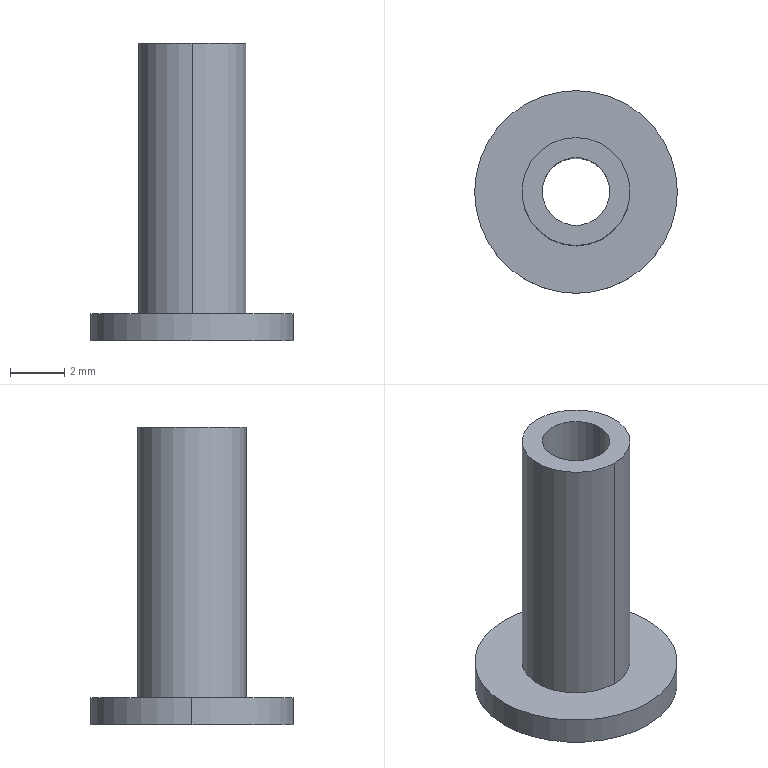Part | STEP file | High-temperature rubber spring guide shaft | 1 solid | 9 faces | box 7.5 x 7.5 x 11 mm | volume 115.846 mm3 | cylinder 6 | plane 3 | commonest cylinder face diameters 2.5 x2 4 x2 7.5 x2
STEP:
#1=CARTESIAN_POINT('',(0.,0.,0.));
#2=DIRECTION('',(0.,0.,1.));
#3=DIRECTION('',(1.,0.,0.));
#4=AXIS2_PLACEMENT_3D('',#1,#2,#3);
#5=CARTESIAN_POINT('',(-3.75,0.,-11.));
#6=VERTEX_POINT('',#5);
#7=CARTESIAN_POINT('',(3.75,0.,-11.));
#8=VERTEX_POINT('',#7);
#9=CARTESIAN_POINT('',(0.,0.,-11.));
#10=DIRECTION('',(0.,0.,-1.));
#11=DIRECTION('',(1.,0.,0.));
#12=AXIS2_PLACEMENT_3D('',#9,#10,#11);
#13=CIRCLE('',#12,3.75);
#14=CARTESIAN_POINT('',(0.,0.,-11.));
#15=DIRECTION('',(0.,0.,1.));
#16=DIRECTION('',(1.,0.,0.));
#17=AXIS2_PLACEMENT_3D('',#14,#15,#16);
#18=CYLINDRICAL_SURFACE('',#17,3.75);
#19=CARTESIAN_POINT('',(6.283,0.));
#20=DIRECTION('',(-1.,0.));
#21=VECTOR('',#20,1.);
#22=LINE('',#19,#21);
#23=(GEOMETRIC_REPRESENTATION_CONTEXT(2)PARAMETRIC_REPRESENTATION_CONTEXT()REPRESENTATION_CONTEXT('',''));
#24=DEFINITIONAL_REPRESENTATION('',(#22),#23);
#25=PCURVE('',#18,#24);
#26=CARTESIAN_POINT('',(-3.795,-3.795,-11.));
#27=DIRECTION('',(0.,0.,1.));
#28=DIRECTION('',(1.,0.,0.));
#29=AXIS2_PLACEMENT_3D('',#26,#27,#28);
#30=PLANE('',#29);
#31=CARTESIAN_POINT('',(7.545,3.795));
#32=CARTESIAN_POINT('',(7.545,-2.7));
#33=CARTESIAN_POINT('',(1.92,0.5474));
#34=CARTESIAN_POINT('',(-3.705,3.795));
#35=CARTESIAN_POINT('',(1.92,7.043));
#36=CARTESIAN_POINT('',(7.545,10.29));
#37=CARTESIAN_POINT('',(7.545,3.795));
#38=(BOUNDED_CURVE()B_SPLINE_CURVE(2,(#31,#32,#33,#34,#35,#36,#37),.UNSPECIFIED.,.T.,.F.)B_SPLINE_CURVE_WITH_KNOTS((1,2,2,2,2,1),(-2.094,0.,2.094,4.189,6.283,8.378),.UNSPECIFIED.)CURVE()GEOMETRIC_REPRESENTATION_ITEM()RATIONAL_B_SPLINE_CURVE((1.,0.5,1.,0.5,1.,0.5,1.))REPRESENTATION_ITEM(''));
#39=(GEOMETRIC_REPRESENTATION_CONTEXT(2)PARAMETRIC_REPRESENTATION_CONTEXT()REPRESENTATION_CONTEXT('',''));
#40=DEFINITIONAL_REPRESENTATION('',(#38),#39);
#41=PCURVE('',#30,#40);
#42=SURFACE_CURVE('',#13,(#25,#41),.PCURVE_S1.);
#43=EDGE_CURVE('',#6,#8,#42,.T.);
#44=ORIENTED_EDGE('',*,*,#43,.F.);
#45=CARTESIAN_POINT('',(-3.75,0.,-10.));
#46=VERTEX_POINT('',#45);
#47=CARTESIAN_POINT('',(-3.75,0.,-11.));
#48=DIRECTION('',(0.,0.,1.));
#49=VECTOR('',#48,1.);
#50=LINE('',#47,#49);
#51=CARTESIAN_POINT('',(3.142,0.));
#52=DIRECTION('',(0.,1.));
#53=VECTOR('',#52,1.);
#54=LINE('',#51,#53);
#55=(GEOMETRIC_REPRESENTATION_CONTEXT(2)PARAMETRIC_REPRESENTATION_CONTEXT()REPRESENTATION_CONTEXT('',''));
#56=DEFINITIONAL_REPRESENTATION('',(#54),#55);
#57=PCURVE('',#18,#56);
#58=CARTESIAN_POINT('',(0.,0.,-11.));
#59=DIRECTION('',(0.,0.,1.));
#60=DIRECTION('',(1.,0.,0.));
#61=AXIS2_PLACEMENT_3D('',#58,#59,#60);
#62=CYLINDRICAL_SURFACE('',#61,3.75);
#63=CARTESIAN_POINT('',(3.142,0.));
#64=DIRECTION('',(0.,1.));
#65=VECTOR('',#64,1.);
#66=LINE('',#63,#65);
#67=(GEOMETRIC_REPRESENTATION_CONTEXT(2)PARAMETRIC_REPRESENTATION_CONTEXT()REPRESENTATION_CONTEXT('',''));
#68=DEFINITIONAL_REPRESENTATION('',(#66),#67);
#69=PCURVE('',#62,#68);
#70=SURFACE_CURVE('',#50,(#57,#69),.PCURVE_S1.);
#71=EDGE_CURVE('',#6,#46,#70,.T.);
#72=ORIENTED_EDGE('',*,*,#71,.T.);
#73=CARTESIAN_POINT('',(3.75,0.,-10.));
#74=VERTEX_POINT('',#73);
#75=CARTESIAN_POINT('',(0.,0.,-10.));
#76=DIRECTION('',(0.,0.,1.));
#77=DIRECTION('',(1.,0.,0.));
#78=AXIS2_PLACEMENT_3D('',#75,#76,#77);
#79=CIRCLE('',#78,3.75);
#80=CARTESIAN_POINT('',(0.,1.));
#81=DIRECTION('',(1.,0.));
#82=VECTOR('',#81,1.);
#83=LINE('',#80,#82);
#84=(GEOMETRIC_REPRESENTATION_CONTEXT(2)PARAMETRIC_REPRESENTATION_CONTEXT()REPRESENTATION_CONTEXT('',''));
#85=DEFINITIONAL_REPRESENTATION('',(#83),#84);
#86=PCURVE('',#18,#85);
#87=CARTESIAN_POINT('',(3.795,-3.795,-10.));
#88=DIRECTION('',(0.,0.,-1.));
#89=DIRECTION('',(-1.,0.,0.));
#90=AXIS2_PLACEMENT_3D('',#87,#88,#89);
#91=PLANE('',#90);
#92=CARTESIAN_POINT('',(0.045,3.795));
#93=CARTESIAN_POINT('',(0.045,10.29));
#94=CARTESIAN_POINT('',(5.67,7.043));
#95=CARTESIAN_POINT('',(11.295,3.795));
#96=CARTESIAN_POINT('',(5.67,0.5474));
#97=CARTESIAN_POINT('',(0.045,-2.7));
#98=CARTESIAN_POINT('',(0.045,3.795));
#99=(BOUNDED_CURVE()B_SPLINE_CURVE(2,(#92,#93,#94,#95,#96,#97,#98),.UNSPECIFIED.,.T.,.F.)B_SPLINE_CURVE_WITH_KNOTS((1,2,2,2,2,1),(-2.094,0.,2.094,4.189,6.283,8.378),.UNSPECIFIED.)CURVE()GEOMETRIC_REPRESENTATION_ITEM()RATIONAL_B_SPLINE_CURVE((1.,0.5,1.,0.5,1.,0.5,1.))REPRESENTATION_ITEM(''));
#100=(GEOMETRIC_REPRESENTATION_CONTEXT(2)PARAMETRIC_REPRESENTATION_CONTEXT()REPRESENTATION_CONTEXT('',''));
#101=DEFINITIONAL_REPRESENTATION('',(#99),#100);
#102=PCURVE('',#91,#101);
#103=SURFACE_CURVE('',#79,(#86,#102),.PCURVE_S1.);
#104=EDGE_CURVE('',#74,#46,#103,.T.);
#105=ORIENTED_EDGE('',*,*,#104,.F.);
#106=CARTESIAN_POINT('',(3.75,0.,-11.));
#107=DIRECTION('',(0.,0.,1.));
#108=VECTOR('',#107,1.);
#109=LINE('',#106,#108);
#110=CARTESIAN_POINT('',(0.,0.));
#111=DIRECTION('',(0.,1.));
#112=VECTOR('',#111,1.);
#113=LINE('',#110,#112);
#114=(GEOMETRIC_REPRESENTATION_CONTEXT(2)PARAMETRIC_REPRESENTATION_CONTEXT()REPRESENTATION_CONTEXT('',''));
#115=DEFINITIONAL_REPRESENTATION('',(#113),#114);
#116=PCURVE('',#18,#115);
#117=CARTESIAN_POINT('',(6.283,0.));
#118=DIRECTION('',(0.,1.));
#119=VECTOR('',#118,1.);
#120=LINE('',#117,#119);
#121=(GEOMETRIC_REPRESENTATION_CONTEXT(2)PARAMETRIC_REPRESENTATION_CONTEXT()REPRESENTATION_CONTEXT('',''));
#122=DEFINITIONAL_REPRESENTATION('',(#120),#121);
#123=PCURVE('',#62,#122);
#124=SURFACE_CURVE('',#109,(#116,#123),.PCURVE_S1.);
#125=EDGE_CURVE('',#8,#74,#124,.T.);
#126=ORIENTED_EDGE('',*,*,#125,.F.);
#127=EDGE_LOOP('',(#44,#72,#105,#126));
#128=FACE_BOUND('',#127,.T.);
#129=ADVANCED_FACE('',(#128),#18,.T.);
#130=CARTESIAN_POINT('',(1.25,0.,-11.));
#131=VERTEX_POINT('',#130);
#132=CARTESIAN_POINT('',(1.25,0.,0.));
#133=VERTEX_POINT('',#132);
#134=CARTESIAN_POINT('',(1.25,0.,-11.));
#135=DIRECTION('',(0.,0.,1.));
#136=VECTOR('',#135,1.);
#137=LINE('',#134,#136);
#138=CARTESIAN_POINT('',(0.,0.,-11.));
#139=DIRECTION('',(0.,0.,1.));
#140=DIRECTION('',(1.,0.,0.));
#141=AXIS2_PLACEMENT_3D('',#138,#139,#140);
#142=CYLINDRICAL_SURFACE('',#141,1.25);
#143=CARTESIAN_POINT('',(6.283,0.));
#144=DIRECTION('',(0.,1.));
#145=VECTOR('',#144,1.);
#146=LINE('',#143,#145);
#147=(GEOMETRIC_REPRESENTATION_CONTEXT(2)PARAMETRIC_REPRESENTATION_CONTEXT()REPRESENTATION_CONTEXT('',''));
#148=DEFINITIONAL_REPRESENTATION('',(#146),#147);
#149=PCURVE('',#142,#148);
#150=CARTESIAN_POINT('',(0.,0.,-11.));
#151=DIRECTION('',(0.,0.,1.));
#152=DIRECTION('',(1.,0.,0.));
#153=AXIS2_PLACEMENT_3D('',#150,#151,#152);
#154=CYLINDRICAL_SURFACE('',#153,1.25);
#155=CARTESIAN_POINT('',(0.,0.));
#156=DIRECTION('',(0.,1.));
#157=VECTOR('',#156,1.);
#158=LINE('',#155,#157);
#159=(GEOMETRIC_REPRESENTATION_CONTEXT(2)PARAMETRIC_REPRESENTATION_CONTEXT()REPRESENTATION_CONTEXT('',''));
#160=DEFINITIONAL_REPRESENTATION('',(#158),#159);
#161=PCURVE('',#154,#160);
#162=SURFACE_CURVE('',#137,(#149,#161),.PCURVE_S1.);
#163=EDGE_CURVE('',#131,#133,#162,.T.);
#164=ORIENTED_EDGE('',*,*,#163,.T.);
#165=CARTESIAN_POINT('',(-1.25,0.,0.));
#166=VERTEX_POINT('',#165);
#167=CARTESIAN_POINT('',(0.,0.,0.));
#168=DIRECTION('',(0.,0.,1.));
#169=DIRECTION('',(1.,0.,0.));
#170=AXIS2_PLACEMENT_3D('',#167,#168,#169);
#171=CIRCLE('',#170,1.25);
#172=CARTESIAN_POINT('',(0.,11.));
#173=DIRECTION('',(1.,0.));
#174=VECTOR('',#173,1.);
#175=LINE('',#172,#174);
#176=(GEOMETRIC_REPRESENTATION_CONTEXT(2)PARAMETRIC_REPRESENTATION_CONTEXT()REPRESENTATION_CONTEXT('',''));
#177=DEFINITIONAL_REPRESENTATION('',(#175),#176);
#178=PCURVE('',#142,#177);
#179=CARTESIAN_POINT('',(2.024,-2.024,0.));
#180=DIRECTION('',(0.,0.,-1.));
#181=DIRECTION('',(-1.,0.,0.));
#182=AXIS2_PLACEMENT_3D('',#179,#180,#181);
#183=PLANE('',#182);
#184=CARTESIAN_POINT('',(0.774,2.024));
#185=CARTESIAN_POINT('',(0.774,4.189));
#186=CARTESIAN_POINT('',(2.649,3.107));
#187=CARTESIAN_POINT('',(4.524,2.024));
#188=CARTESIAN_POINT('',(2.649,0.9415));
#189=CARTESIAN_POINT('',(0.774,-0.1411));
#190=CARTESIAN_POINT('',(0.774,2.024));
#191=(BOUNDED_CURVE()B_SPLINE_CURVE(2,(#184,#185,#186,#187,#188,#189,#190),.UNSPECIFIED.,.T.,.F.)B_SPLINE_CURVE_WITH_KNOTS((1,2,2,2,2,1),(-2.094,0.,2.094,4.189,6.283,8.378),.UNSPECIFIED.)CURVE()GEOMETRIC_REPRESENTATION_ITEM()RATIONAL_B_SPLINE_CURVE((1.,0.5,1.,0.5,1.,0.5,1.))REPRESENTATION_ITEM(''));
#192=(GEOMETRIC_REPRESENTATION_CONTEXT(2)PARAMETRIC_REPRESENTATION_CONTEXT()REPRESENTATION_CONTEXT('',''));
#193=DEFINITIONAL_REPRESENTATION('',(#191),#192);
#194=PCURVE('',#183,#193);
#195=SURFACE_CURVE('',#171,(#178,#194),.PCURVE_S1.);
#196=EDGE_CURVE('',#166,#133,#195,.T.);
#197=ORIENTED_EDGE('',*,*,#196,.F.);
#198=CARTESIAN_POINT('',(-1.25,0.,-11.));
#199=VERTEX_POINT('',#198);
#200=CARTESIAN_POINT('',(-1.25,0.,-11.));
#201=DIRECTION('',(0.,0.,1.));
#202=VECTOR('',#201,1.);
#203=LINE('',#200,#202);
#204=CARTESIAN_POINT('',(3.142,0.));
#205=DIRECTION('',(0.,1.));
#206=VECTOR('',#205,1.);
#207=LINE('',#204,#206);
#208=(GEOMETRIC_REPRESENTATION_CONTEXT(2)PARAMETRIC_REPRESENTATION_CONTEXT()REPRESENTATION_CONTEXT('',''));
#209=DEFINITIONAL_REPRESENTATION('',(#207),#208);
#210=PCURVE('',#142,#209);
#211=CARTESIAN_POINT('',(3.142,0.));
#212=DIRECTION('',(0.,1.));
#213=VECTOR('',#212,1.);
#214=LINE('',#211,#213);
#215=(GEOMETRIC_REPRESENTATION_CONTEXT(2)PARAMETRIC_REPRESENTATION_CONTEXT()REPRESENTATION_CONTEXT('',''));
#216=DEFINITIONAL_REPRESENTATION('',(#214),#215);
#217=PCURVE('',#154,#216);
#218=SURFACE_CURVE('',#203,(#210,#217),.PCURVE_S1.);
#219=EDGE_CURVE('',#199,#166,#218,.T.);
#220=ORIENTED_EDGE('',*,*,#219,.F.);
#221=CARTESIAN_POINT('',(0.,0.,-11.));
#222=DIRECTION('',(0.,0.,-1.));
#223=DIRECTION('',(1.,0.,0.));
#224=AXIS2_PLACEMENT_3D('',#221,#222,#223);
#225=CIRCLE('',#224,1.25);
#226=CARTESIAN_POINT('',(6.283,0.));
#227=DIRECTION('',(-1.,0.));
#228=VECTOR('',#227,1.);
#229=LINE('',#226,#228);
#230=(GEOMETRIC_REPRESENTATION_CONTEXT(2)PARAMETRIC_REPRESENTATION_CONTEXT()REPRESENTATION_CONTEXT('',''));
#231=DEFINITIONAL_REPRESENTATION('',(#229),#230);
#232=PCURVE('',#142,#231);
#233=CARTESIAN_POINT('',(5.045,3.795));
#234=CARTESIAN_POINT('',(5.045,1.63));
#235=CARTESIAN_POINT('',(3.17,2.712));
#236=CARTESIAN_POINT('',(1.295,3.795));
#237=CARTESIAN_POINT('',(3.17,4.878));
#238=CARTESIAN_POINT('',(5.045,5.96));
#239=CARTESIAN_POINT('',(5.045,3.795));
#240=(BOUNDED_CURVE()B_SPLINE_CURVE(2,(#233,#234,#235,#236,#237,#238,#239),.UNSPECIFIED.,.T.,.F.)B_SPLINE_CURVE_WITH_KNOTS((1,2,2,2,2,1),(-2.094,0.,2.094,4.189,6.283,8.378),.UNSPECIFIED.)CURVE()GEOMETRIC_REPRESENTATION_ITEM()RATIONAL_B_SPLINE_CURVE((1.,0.5,1.,0.5,1.,0.5,1.))REPRESENTATION_ITEM(''));
#241=(GEOMETRIC_REPRESENTATION_CONTEXT(2)PARAMETRIC_REPRESENTATION_CONTEXT()REPRESENTATION_CONTEXT('',''));
#242=DEFINITIONAL_REPRESENTATION('',(#240),#241);
#243=PCURVE('',#30,#242);
#244=SURFACE_CURVE('',#225,(#232,#243),.PCURVE_S1.);
#245=EDGE_CURVE('',#131,#199,#244,.T.);
#246=ORIENTED_EDGE('',*,*,#245,.F.);
#247=EDGE_LOOP('',(#164,#197,#220,#246));
#248=FACE_BOUND('',#247,.F.);
#249=ADVANCED_FACE('',(#248),#142,.F.);
#250=CARTESIAN_POINT('',(0.,-2.,-10.));
#251=VERTEX_POINT('',#250);
#252=CARTESIAN_POINT('',(0.,2.,-10.));
#253=VERTEX_POINT('',#252);
#254=CARTESIAN_POINT('',(0.,0.,-10.));
#255=DIRECTION('',(0.,0.,1.));
#256=DIRECTION('',(0.,-1.,0.));
#257=AXIS2_PLACEMENT_3D('',#254,#255,#256);
#258=CIRCLE('',#257,2.);
#259=CARTESIAN_POINT('',(0.,0.,-10.));
#260=DIRECTION('',(0.,0.,1.));
#261=DIRECTION('',(0.,-1.,0.));
#262=AXIS2_PLACEMENT_3D('',#259,#260,#261);
#263=CYLINDRICAL_SURFACE('',#262,2.);
#264=CARTESIAN_POINT('',(0.,0.));
#265=DIRECTION('',(1.,0.));
#266=VECTOR('',#265,1.);
#267=LINE('',#264,#266);
#268=(GEOMETRIC_REPRESENTATION_CONTEXT(2)PARAMETRIC_REPRESENTATION_CONTEXT()REPRESENTATION_CONTEXT('',''));
#269=DEFINITIONAL_REPRESENTATION('',(#267),#268);
#270=PCURVE('',#263,#269);
#271=CARTESIAN_POINT('',(3.795,1.795));
#272=CARTESIAN_POINT('',(0.3309,1.795));
#273=CARTESIAN_POINT('',(2.063,4.795));
#274=CARTESIAN_POINT('',(3.795,7.795));
#275=CARTESIAN_POINT('',(5.527,4.795));
#276=CARTESIAN_POINT('',(7.259,1.795));
#277=CARTESIAN_POINT('',(3.795,1.795));
#278=(BOUNDED_CURVE()B_SPLINE_CURVE(2,(#271,#272,#273,#274,#275,#276,#277),.UNSPECIFIED.,.T.,.F.)B_SPLINE_CURVE_WITH_KNOTS((1,2,2,2,2,1),(-2.094,0.,2.094,4.189,6.283,8.378),.UNSPECIFIED.)CURVE()GEOMETRIC_REPRESENTATION_ITEM()RATIONAL_B_SPLINE_CURVE((1.,0.5,1.,0.5,1.,0.5,1.))REPRESENTATION_ITEM(''));
#279=(GEOMETRIC_REPRESENTATION_CONTEXT(2)PARAMETRIC_REPRESENTATION_CONTEXT()REPRESENTATION_CONTEXT('',''));
#280=DEFINITIONAL_REPRESENTATION('',(#278),#279);
#281=PCURVE('',#91,#280);
#282=SURFACE_CURVE('',#258,(#270,#281),.PCURVE_S1.);
#283=EDGE_CURVE('',#251,#253,#282,.T.);
#284=ORIENTED_EDGE('',*,*,#283,.T.);
#285=CARTESIAN_POINT('',(0.,2.,0.));
#286=VERTEX_POINT('',#285);
#287=CARTESIAN_POINT('',(0.,2.,-10.));
#288=DIRECTION('',(0.,0.,1.));
#289=VECTOR('',#288,1.);
#290=LINE('',#287,#289);
#291=CARTESIAN_POINT('',(3.142,0.));
#292=DIRECTION('',(0.,1.));
#293=VECTOR('',#292,1.);
#294=LINE('',#291,#293);
#295=(GEOMETRIC_REPRESENTATION_CONTEXT(2)PARAMETRIC_REPRESENTATION_CONTEXT()REPRESENTATION_CONTEXT('',''));
#296=DEFINITIONAL_REPRESENTATION('',(#294),#295);
#297=PCURVE('',#263,#296);
#298=CARTESIAN_POINT('',(0.,0.,-10.));
#299=DIRECTION('',(0.,0.,1.));
#300=DIRECTION('',(0.,-1.,0.));
#301=AXIS2_PLACEMENT_3D('',#298,#299,#300);
#302=CYLINDRICAL_SURFACE('',#301,2.);
#303=CARTESIAN_POINT('',(3.142,0.));
#304=DIRECTION('',(0.,1.));
#305=VECTOR('',#304,1.);
#306=LINE('',#303,#305);
#307=(GEOMETRIC_REPRESENTATION_CONTEXT(2)PARAMETRIC_REPRESENTATION_CONTEXT()REPRESENTATION_CONTEXT('',''));
#308=DEFINITIONAL_REPRESENTATION('',(#306),#307);
#309=PCURVE('',#302,#308);
#310=SURFACE_CURVE('',#290,(#297,#309),.PCURVE_S1.);
#311=EDGE_CURVE('',#253,#286,#310,.T.);
#312=ORIENTED_EDGE('',*,*,#311,.T.);
#313=CARTESIAN_POINT('',(0.,-2.,0.));
#314=VERTEX_POINT('',#313);
#315=CARTESIAN_POINT('',(0.,0.,0.));
#316=DIRECTION('',(0.,0.,1.));
#317=DIRECTION('',(0.,-1.,0.));
#318=AXIS2_PLACEMENT_3D('',#315,#316,#317);
#319=CIRCLE('',#318,2.);
#320=CARTESIAN_POINT('',(0.,10.));
#321=DIRECTION('',(1.,0.));
#322=VECTOR('',#321,1.);
#323=LINE('',#320,#322);
#324=(GEOMETRIC_REPRESENTATION_CONTEXT(2)PARAMETRIC_REPRESENTATION_CONTEXT()REPRESENTATION_CONTEXT('',''));
#325=DEFINITIONAL_REPRESENTATION('',(#323),#324);
#326=PCURVE('',#263,#325);
#327=CARTESIAN_POINT('',(2.024,0.024));
#328=CARTESIAN_POINT('',(-1.44,0.024));
#329=CARTESIAN_POINT('',(0.2919,3.024));
#330=CARTESIAN_POINT('',(2.024,6.024));
#331=CARTESIAN_POINT('',(3.756,3.024));
#332=CARTESIAN_POINT('',(5.488,0.024));
#333=CARTESIAN_POINT('',(2.024,0.024));
#334=(BOUNDED_CURVE()B_SPLINE_CURVE(2,(#327,#328,#329,#330,#331,#332,#333),.UNSPECIFIED.,.T.,.F.)B_SPLINE_CURVE_WITH_KNOTS((1,2,2,2,2,1),(-2.094,0.,2.094,4.189,6.283,8.378),.UNSPECIFIED.)CURVE()GEOMETRIC_REPRESENTATION_ITEM()RATIONAL_B_SPLINE_CURVE((1.,0.5,1.,0.5,1.,0.5,1.))REPRESENTATION_ITEM(''));
#335=(GEOMETRIC_REPRESENTATION_CONTEXT(2)PARAMETRIC_REPRESENTATION_CONTEXT()REPRESENTATION_CONTEXT('',''));
#336=DEFINITIONAL_REPRESENTATION('',(#334),#335);
#337=PCURVE('',#183,#336);
#338=SURFACE_CURVE('',#319,(#326,#337),.PCURVE_S1.);
#339=EDGE_CURVE('',#314,#286,#338,.T.);
#340=ORIENTED_EDGE('',*,*,#339,.F.);
#341=CARTESIAN_POINT('',(0.,-2.,-10.));
#342=DIRECTION('',(0.,0.,1.));
#343=VECTOR('',#342,1.);
#344=LINE('',#341,#343);
#345=CARTESIAN_POINT('',(0.,0.));
#346=DIRECTION('',(0.,1.));
#347=VECTOR('',#346,1.);
#348=LINE('',#345,#347);
#349=(GEOMETRIC_REPRESENTATION_CONTEXT(2)PARAMETRIC_REPRESENTATION_CONTEXT()REPRESENTATION_CONTEXT('',''));
#350=DEFINITIONAL_REPRESENTATION('',(#348),#349);
#351=PCURVE('',#263,#350);
#352=CARTESIAN_POINT('',(6.283,0.));
#353=DIRECTION('',(0.,1.));
#354=VECTOR('',#353,1.);
#355=LINE('',#352,#354);
#356=(GEOMETRIC_REPRESENTATION_CONTEXT(2)PARAMETRIC_REPRESENTATION_CONTEXT()REPRESENTATION_CONTEXT('',''));
#357=DEFINITIONAL_REPRESENTATION('',(#355),#356);
#358=PCURVE('',#302,#357);
#359=SURFACE_CURVE('',#344,(#351,#358),.PCURVE_S1.);
#360=EDGE_CURVE('',#251,#314,#359,.T.);
#361=ORIENTED_EDGE('',*,*,#360,.F.);
#362=EDGE_LOOP('',(#284,#312,#340,#361));
#363=FACE_BOUND('',#362,.T.);
#364=ADVANCED_FACE('',(#363),#263,.T.);
#365=ORIENTED_EDGE('',*,*,#71,.F.);
#366=CARTESIAN_POINT('',(0.,0.,-11.));
#367=DIRECTION('',(0.,0.,-1.));
#368=DIRECTION('',(1.,0.,0.));
#369=AXIS2_PLACEMENT_3D('',#366,#367,#368);
#370=CIRCLE('',#369,3.75);
#371=CARTESIAN_POINT('',(6.283,0.));
#372=DIRECTION('',(-1.,0.));
#373=VECTOR('',#372,1.);
#374=LINE('',#371,#373);
#375=(GEOMETRIC_REPRESENTATION_CONTEXT(2)PARAMETRIC_REPRESENTATION_CONTEXT()REPRESENTATION_CONTEXT('',''));
#376=DEFINITIONAL_REPRESENTATION('',(#374),#375);
#377=PCURVE('',#62,#376);
#378=CARTESIAN_POINT('',(7.545,3.795));
#379=CARTESIAN_POINT('',(7.545,-2.7));
#380=CARTESIAN_POINT('',(1.92,0.5474));
#381=CARTESIAN_POINT('',(-3.705,3.795));
#382=CARTESIAN_POINT('',(1.92,7.043));
#383=CARTESIAN_POINT('',(7.545,10.29));
#384=CARTESIAN_POINT('',(7.545,3.795));
#385=(BOUNDED_CURVE()B_SPLINE_CURVE(2,(#378,#379,#380,#381,#382,#383,#384),.UNSPECIFIED.,.T.,.F.)B_SPLINE_CURVE_WITH_KNOTS((1,2,2,2,2,1),(-2.094,0.,2.094,4.189,6.283,8.378),.UNSPECIFIED.)CURVE()GEOMETRIC_REPRESENTATION_ITEM()RATIONAL_B_SPLINE_CURVE((1.,0.5,1.,0.5,1.,0.5,1.))REPRESENTATION_ITEM(''));
#386=(GEOMETRIC_REPRESENTATION_CONTEXT(2)PARAMETRIC_REPRESENTATION_CONTEXT()REPRESENTATION_CONTEXT('',''));
#387=DEFINITIONAL_REPRESENTATION('',(#385),#386);
#388=PCURVE('',#30,#387);
#389=SURFACE_CURVE('',#370,(#377,#388),.PCURVE_S1.);
#390=EDGE_CURVE('',#8,#6,#389,.T.);
#391=ORIENTED_EDGE('',*,*,#390,.F.);
#392=ORIENTED_EDGE('',*,*,#125,.T.);
#393=CARTESIAN_POINT('',(0.,0.,-10.));
#394=DIRECTION('',(0.,0.,1.));
#395=DIRECTION('',(1.,0.,0.));
#396=AXIS2_PLACEMENT_3D('',#393,#394,#395);
#397=CIRCLE('',#396,3.75);
#398=CARTESIAN_POINT('',(0.,1.));
#399=DIRECTION('',(1.,0.));
#400=VECTOR('',#399,1.);
#401=LINE('',#398,#400);
#402=(GEOMETRIC_REPRESENTATION_CONTEXT(2)PARAMETRIC_REPRESENTATION_CONTEXT()REPRESENTATION_CONTEXT('',''));
#403=DEFINITIONAL_REPRESENTATION('',(#401),#402);
#404=PCURVE('',#62,#403);
#405=CARTESIAN_POINT('',(0.045,3.795));
#406=CARTESIAN_POINT('',(0.045,10.29));
#407=CARTESIAN_POINT('',(5.67,7.043));
#408=CARTESIAN_POINT('',(11.295,3.795));
#409=CARTESIAN_POINT('',(5.67,0.5474));
#410=CARTESIAN_POINT('',(0.045,-2.7));
#411=CARTESIAN_POINT('',(0.045,3.795));
#412=(BOUNDED_CURVE()B_SPLINE_CURVE(2,(#405,#406,#407,#408,#409,#410,#411),.UNSPECIFIED.,.T.,.F.)B_SPLINE_CURVE_WITH_KNOTS((1,2,2,2,2,1),(-2.094,0.,2.094,4.189,6.283,8.378),.UNSPECIFIED.)CURVE()GEOMETRIC_REPRESENTATION_ITEM()RATIONAL_B_SPLINE_CURVE((1.,0.5,1.,0.5,1.,0.5,1.))REPRESENTATION_ITEM(''));
#413=(GEOMETRIC_REPRESENTATION_CONTEXT(2)PARAMETRIC_REPRESENTATION_CONTEXT()REPRESENTATION_CONTEXT('',''));
#414=DEFINITIONAL_REPRESENTATION('',(#412),#413);
#415=PCURVE('',#91,#414);
#416=SURFACE_CURVE('',#397,(#404,#415),.PCURVE_S1.);
#417=EDGE_CURVE('',#46,#74,#416,.T.);
#418=ORIENTED_EDGE('',*,*,#417,.F.);
#419=EDGE_LOOP('',(#365,#391,#392,#418));
#420=FACE_BOUND('',#419,.T.);
#421=ADVANCED_FACE('',(#420),#62,.T.);
#422=ORIENTED_EDGE('',*,*,#245,.F.);
#423=CARTESIAN_POINT('',(0.,0.,-11.));
#424=DIRECTION('',(0.,0.,-1.));
#425=DIRECTION('',(1.,0.,0.));
#426=AXIS2_PLACEMENT_3D('',#423,#424,#425);
#427=CIRCLE('',#426,1.25);
#428=CARTESIAN_POINT('',(5.045,3.795));
#429=CARTESIAN_POINT('',(5.045,1.63));
#430=CARTESIAN_POINT('',(3.17,2.712));
#431=CARTESIAN_POINT('',(1.295,3.795));
#432=CARTESIAN_POINT('',(3.17,4.878));
#433=CARTESIAN_POINT('',(5.045,5.96));
#434=CARTESIAN_POINT('',(5.045,3.795));
#435=(BOUNDED_CURVE()B_SPLINE_CURVE(2,(#428,#429,#430,#431,#432,#433,#434),.UNSPECIFIED.,.T.,.F.)B_SPLINE_CURVE_WITH_KNOTS((1,2,2,2,2,1),(-2.094,0.,2.094,4.189,6.283,8.378),.UNSPECIFIED.)CURVE()GEOMETRIC_REPRESENTATION_ITEM()RATIONAL_B_SPLINE_CURVE((1.,0.5,1.,0.5,1.,0.5,1.))REPRESENTATION_ITEM(''));
#436=(GEOMETRIC_REPRESENTATION_CONTEXT(2)PARAMETRIC_REPRESENTATION_CONTEXT()REPRESENTATION_CONTEXT('',''));
#437=DEFINITIONAL_REPRESENTATION('',(#435),#436);
#438=PCURVE('',#30,#437);
#439=CARTESIAN_POINT('',(6.283,0.));
#440=DIRECTION('',(-1.,0.));
#441=VECTOR('',#440,1.);
#442=LINE('',#439,#441);
#443=(GEOMETRIC_REPRESENTATION_CONTEXT(2)PARAMETRIC_REPRESENTATION_CONTEXT()REPRESENTATION_CONTEXT('',''));
#444=DEFINITIONAL_REPRESENTATION('',(#442),#443);
#445=PCURVE('',#154,#444);
#446=SURFACE_CURVE('',#427,(#438,#445),.PCURVE_S1.);
#447=EDGE_CURVE('',#199,#131,#446,.T.);
#448=ORIENTED_EDGE('',*,*,#447,.F.);
#449=EDGE_LOOP('',(#422,#448));
#450=FACE_BOUND('',#449,.T.);
#451=ORIENTED_EDGE('',*,*,#390,.T.);
#452=ORIENTED_EDGE('',*,*,#43,.T.);
#453=EDGE_LOOP('',(#451,#452));
#454=FACE_BOUND('',#453,.T.);
#455=ADVANCED_FACE('',(#450,#454),#30,.F.);
#456=ORIENTED_EDGE('',*,*,#283,.F.);
#457=CARTESIAN_POINT('',(0.,0.,-10.));
#458=DIRECTION('',(0.,0.,1.));
#459=DIRECTION('',(0.,-1.,0.));
#460=AXIS2_PLACEMENT_3D('',#457,#458,#459);
#461=CIRCLE('',#460,2.);
#462=CARTESIAN_POINT('',(3.795,1.795));
#463=CARTESIAN_POINT('',(0.3309,1.795));
#464=CARTESIAN_POINT('',(2.063,4.795));
#465=CARTESIAN_POINT('',(3.795,7.795));
#466=CARTESIAN_POINT('',(5.527,4.795));
#467=CARTESIAN_POINT('',(7.259,1.795));
#468=CARTESIAN_POINT('',(3.795,1.795));
#469=(BOUNDED_CURVE()B_SPLINE_CURVE(2,(#462,#463,#464,#465,#466,#467,#468),.UNSPECIFIED.,.T.,.F.)B_SPLINE_CURVE_WITH_KNOTS((1,2,2,2,2,1),(-2.094,0.,2.094,4.189,6.283,8.378),.UNSPECIFIED.)CURVE()GEOMETRIC_REPRESENTATION_ITEM()RATIONAL_B_SPLINE_CURVE((1.,0.5,1.,0.5,1.,0.5,1.))REPRESENTATION_ITEM(''));
#470=(GEOMETRIC_REPRESENTATION_CONTEXT(2)PARAMETRIC_REPRESENTATION_CONTEXT()REPRESENTATION_CONTEXT('',''));
#471=DEFINITIONAL_REPRESENTATION('',(#469),#470);
#472=PCURVE('',#91,#471);
#473=CARTESIAN_POINT('',(0.,0.));
#474=DIRECTION('',(1.,0.));
#475=VECTOR('',#474,1.);
#476=LINE('',#473,#475);
#477=(GEOMETRIC_REPRESENTATION_CONTEXT(2)PARAMETRIC_REPRESENTATION_CONTEXT()REPRESENTATION_CONTEXT('',''));
#478=DEFINITIONAL_REPRESENTATION('',(#476),#477);
#479=PCURVE('',#302,#478);
#480=SURFACE_CURVE('',#461,(#472,#479),.PCURVE_S1.);
#481=EDGE_CURVE('',#253,#251,#480,.T.);
#482=ORIENTED_EDGE('',*,*,#481,.F.);
#483=EDGE_LOOP('',(#456,#482));
#484=FACE_BOUND('',#483,.T.);
#485=ORIENTED_EDGE('',*,*,#104,.T.);
#486=ORIENTED_EDGE('',*,*,#417,.T.);
#487=EDGE_LOOP('',(#485,#486));
#488=FACE_BOUND('',#487,.T.);
#489=ADVANCED_FACE('',(#484,#488),#91,.F.);
#490=CARTESIAN_POINT('',(0.,0.,0.));
#491=DIRECTION('',(0.,0.,1.));
#492=DIRECTION('',(1.,0.,0.));
#493=AXIS2_PLACEMENT_3D('',#490,#491,#492);
#494=CIRCLE('',#493,1.25);
#495=CARTESIAN_POINT('',(0.,11.));
#496=DIRECTION('',(1.,0.));
#497=VECTOR('',#496,1.);
#498=LINE('',#495,#497);
#499=(GEOMETRIC_REPRESENTATION_CONTEXT(2)PARAMETRIC_REPRESENTATION_CONTEXT()REPRESENTATION_CONTEXT('',''));
#500=DEFINITIONAL_REPRESENTATION('',(#498),#499);
#501=PCURVE('',#154,#500);
#502=CARTESIAN_POINT('',(0.774,2.024));
#503=CARTESIAN_POINT('',(0.774,4.189));
#504=CARTESIAN_POINT('',(2.649,3.107));
#505=CARTESIAN_POINT('',(4.524,2.024));
#506=CARTESIAN_POINT('',(2.649,0.9415));
#507=CARTESIAN_POINT('',(0.774,-0.1411));
#508=CARTESIAN_POINT('',(0.774,2.024));
#509=(BOUNDED_CURVE()B_SPLINE_CURVE(2,(#502,#503,#504,#505,#506,#507,#508),.UNSPECIFIED.,.T.,.F.)B_SPLINE_CURVE_WITH_KNOTS((1,2,2,2,2,1),(-2.094,0.,2.094,4.189,6.283,8.378),.UNSPECIFIED.)CURVE()GEOMETRIC_REPRESENTATION_ITEM()RATIONAL_B_SPLINE_CURVE((1.,0.5,1.,0.5,1.,0.5,1.))REPRESENTATION_ITEM(''));
#510=(GEOMETRIC_REPRESENTATION_CONTEXT(2)PARAMETRIC_REPRESENTATION_CONTEXT()REPRESENTATION_CONTEXT('',''));
#511=DEFINITIONAL_REPRESENTATION('',(#509),#510);
#512=PCURVE('',#183,#511);
#513=SURFACE_CURVE('',#494,(#501,#512),.PCURVE_S1.);
#514=EDGE_CURVE('',#133,#166,#513,.T.);
#515=ORIENTED_EDGE('',*,*,#514,.F.);
#516=ORIENTED_EDGE('',*,*,#163,.F.);
#517=ORIENTED_EDGE('',*,*,#447,.F.);
#518=ORIENTED_EDGE('',*,*,#219,.T.);
#519=EDGE_LOOP('',(#515,#516,#517,#518));
#520=FACE_BOUND('',#519,.F.);
#521=ADVANCED_FACE('',(#520),#154,.F.);
#522=ORIENTED_EDGE('',*,*,#311,.F.);
#523=ORIENTED_EDGE('',*,*,#481,.T.);
#524=ORIENTED_EDGE('',*,*,#360,.T.);
#525=CARTESIAN_POINT('',(0.,0.,0.));
#526=DIRECTION('',(0.,0.,1.));
#527=DIRECTION('',(0.,-1.,0.));
#528=AXIS2_PLACEMENT_3D('',#525,#526,#527);
#529=CIRCLE('',#528,2.);
#530=CARTESIAN_POINT('',(0.,10.));
#531=DIRECTION('',(1.,0.));
#532=VECTOR('',#531,1.);
#533=LINE('',#530,#532);
#534=(GEOMETRIC_REPRESENTATION_CONTEXT(2)PARAMETRIC_REPRESENTATION_CONTEXT()REPRESENTATION_CONTEXT('',''));
#535=DEFINITIONAL_REPRESENTATION('',(#533),#534);
#536=PCURVE('',#302,#535);
#537=CARTESIAN_POINT('',(2.024,0.024));
#538=CARTESIAN_POINT('',(-1.44,0.024));
#539=CARTESIAN_POINT('',(0.2919,3.024));
#540=CARTESIAN_POINT('',(2.024,6.024));
#541=CARTESIAN_POINT('',(3.756,3.024));
#542=CARTESIAN_POINT('',(5.488,0.024));
#543=CARTESIAN_POINT('',(2.024,0.024));
#544=(BOUNDED_CURVE()B_SPLINE_CURVE(2,(#537,#538,#539,#540,#541,#542,#543),.UNSPECIFIED.,.T.,.F.)B_SPLINE_CURVE_WITH_KNOTS((1,2,2,2,2,1),(-2.094,0.,2.094,4.189,6.283,8.378),.UNSPECIFIED.)CURVE()GEOMETRIC_REPRESENTATION_ITEM()RATIONAL_B_SPLINE_CURVE((1.,0.5,1.,0.5,1.,0.5,1.))REPRESENTATION_ITEM(''));
#545=(GEOMETRIC_REPRESENTATION_CONTEXT(2)PARAMETRIC_REPRESENTATION_CONTEXT()REPRESENTATION_CONTEXT('',''));
#546=DEFINITIONAL_REPRESENTATION('',(#544),#545);
#547=PCURVE('',#183,#546);
#548=SURFACE_CURVE('',#529,(#536,#547),.PCURVE_S1.);
#549=EDGE_CURVE('',#286,#314,#548,.T.);
#550=ORIENTED_EDGE('',*,*,#549,.F.);
#551=EDGE_LOOP('',(#522,#523,#524,#550));
#552=FACE_BOUND('',#551,.T.);
#553=ADVANCED_FACE('',(#552),#302,.T.);
#554=ORIENTED_EDGE('',*,*,#514,.F.);
#555=ORIENTED_EDGE('',*,*,#196,.F.);
#556=EDGE_LOOP('',(#554,#555));
#557=FACE_BOUND('',#556,.T.);
#558=ORIENTED_EDGE('',*,*,#339,.T.);
#559=ORIENTED_EDGE('',*,*,#549,.T.);
#560=EDGE_LOOP('',(#558,#559));
#561=FACE_BOUND('',#560,.T.);
#562=ADVANCED_FACE('',(#557,#561),#183,.F.);
#563=CLOSED_SHELL('',(#129,#249,#364,#421,#455,#489,#521,#553,#562));
#564=MANIFOLD_SOLID_BREP('',#563);
#565=(LENGTH_UNIT()NAMED_UNIT(*)SI_UNIT(.MILLI.,.METRE.));
#566=UNCERTAINTY_MEASURE_WITH_UNIT(LENGTH_MEASURE(0.0000001),#565,'','');
#567=(NAMED_UNIT(*)PLANE_ANGLE_UNIT()SI_UNIT($,.RADIAN.));
#568=(NAMED_UNIT(*)SI_UNIT($,.STERADIAN.)SOLID_ANGLE_UNIT());
#569=(GEOMETRIC_REPRESENTATION_CONTEXT(3)GLOBAL_UNCERTAINTY_ASSIGNED_CONTEXT((#566))GLOBAL_UNIT_ASSIGNED_CONTEXT((#565,#567,#568))REPRESENTATION_CONTEXT('',''));
#570=ADVANCED_BREP_SHAPE_REPRESENTATION('',(#4,#564),#569);